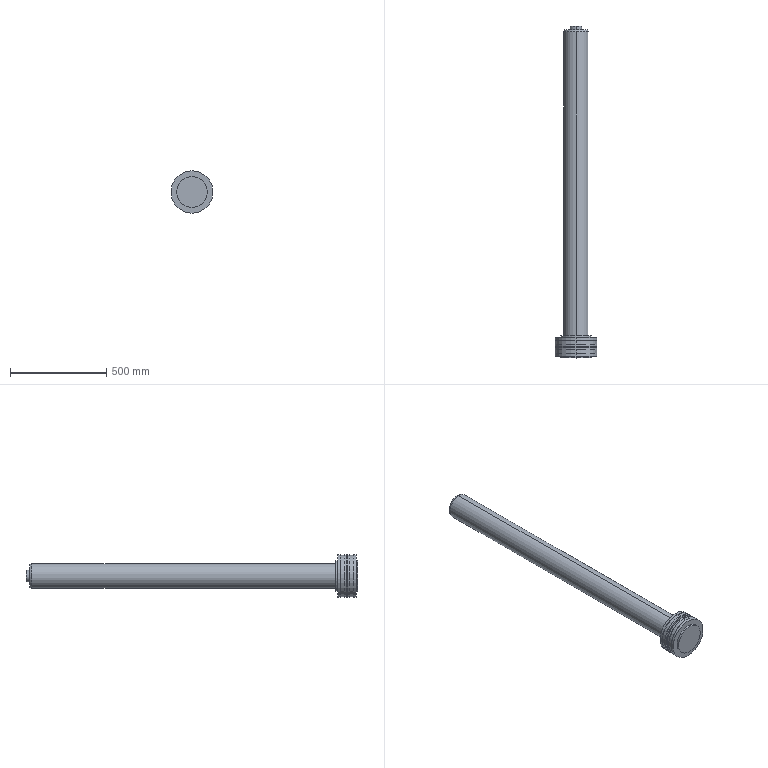Part | SolidWorks | features Revolution 1 | 1 solid | 36 faces | box 220 x 1728 x 220 mm | volume 25109118 mm3 | cylinder 22 | plane 12 | cone 2 | commonest cylinder face diameters 220 x8 160 x4 215 x4 60 x2 130 x2 199 x2
STEP:
#1=CARTESIAN_POINT('',(0.,1728.,-30.));
#2=VERTEX_POINT('',#1);
#3=CARTESIAN_POINT('',(0.,1728.,30.));
#4=VERTEX_POINT('',#3);
#5=CARTESIAN_POINT('',(0.,1728.,0.));
#6=DIRECTION('',(0.,-1.,0.));
#7=DIRECTION('',(0.,0.,-1.));
#8=AXIS2_PLACEMENT_3D('',#5,#6,#7);
#9=CIRCLE('',#8,30.);
#10=EDGE_CURVE('',#2,#4,#9,.T.);
#11=ORIENTED_EDGE('',*,*,#10,.T.);
#12=CARTESIAN_POINT('',(0.,1708.,30.));
#13=VERTEX_POINT('',#12);
#14=CARTESIAN_POINT('',(0.,0.,30.));
#15=DIRECTION('',(0.,-1.,0.));
#16=VECTOR('',#15,1000.);
#17=LINE('',#14,#16);
#18=EDGE_CURVE('',#4,#13,#17,.T.);
#19=ORIENTED_EDGE('',*,*,#18,.T.);
#20=CARTESIAN_POINT('',(0.,1708.,-30.));
#21=VERTEX_POINT('',#20);
#22=CARTESIAN_POINT('',(0.,1708.,0.));
#23=DIRECTION('',(0.,-1.,0.));
#24=DIRECTION('',(0.,0.,-1.));
#25=AXIS2_PLACEMENT_3D('',#22,#23,#24);
#26=CIRCLE('',#25,30.);
#27=EDGE_CURVE('',#21,#13,#26,.T.);
#28=ORIENTED_EDGE('',*,*,#27,.F.);
#29=CARTESIAN_POINT('',(0.,0.,-30.));
#30=DIRECTION('',(0.,-1.,0.));
#31=VECTOR('',#30,1000.);
#32=LINE('',#29,#31);
#33=EDGE_CURVE('',#2,#21,#32,.T.);
#34=ORIENTED_EDGE('',*,*,#33,.F.);
#35=EDGE_LOOP('',(#11,#19,#28,#34));
#36=FACE_OUTER_BOUND('',#35,.T.);
#37=CARTESIAN_POINT('',(0.,0.,0.));
#38=DIRECTION('',(0.,-1.,0.));
#39=DIRECTION('',(0.,0.,-1.));
#40=AXIS2_PLACEMENT_3D('',#37,#38,#39);
#41=CYLINDRICAL_SURFACE('',#40,30.);
#42=ADVANCED_FACE('',(#36),#41,.T.);
#43=CARTESIAN_POINT('',(0.,1708.,-61.36));
#44=VERTEX_POINT('',#43);
#45=CARTESIAN_POINT('',(0.,1708.,61.36));
#46=VERTEX_POINT('',#45);
#47=CARTESIAN_POINT('',(0.,1708.,0.));
#48=DIRECTION('',(0.,-1.,0.));
#49=DIRECTION('',(0.,0.,-1.));
#50=AXIS2_PLACEMENT_3D('',#47,#48,#49);
#51=CIRCLE('',#50,61.36);
#52=EDGE_CURVE('',#44,#46,#51,.T.);
#53=ORIENTED_EDGE('',*,*,#52,.T.);
#54=CARTESIAN_POINT('',(0.,1698.,65.));
#55=VERTEX_POINT('',#54);
#56=CARTESIAN_POINT('',(0.,1698.,65.));
#57=DIRECTION('',(0.,-0.9397,0.342));
#58=VECTOR('',#57,1000.);
#59=LINE('',#56,#58);
#60=EDGE_CURVE('',#46,#55,#59,.T.);
#61=ORIENTED_EDGE('',*,*,#60,.T.);
#62=CARTESIAN_POINT('',(0.,1698.,-65.));
#63=VERTEX_POINT('',#62);
#64=CARTESIAN_POINT('',(0.,1698.,0.));
#65=DIRECTION('',(0.,-1.,0.));
#66=DIRECTION('',(0.,0.,-1.));
#67=AXIS2_PLACEMENT_3D('',#64,#65,#66);
#68=CIRCLE('',#67,65.);
#69=EDGE_CURVE('',#63,#55,#68,.T.);
#70=ORIENTED_EDGE('',*,*,#69,.F.);
#71=CARTESIAN_POINT('',(0.,1698.,-65.));
#72=DIRECTION('',(0.,-0.9397,-0.342));
#73=VECTOR('',#72,1000.);
#74=LINE('',#71,#73);
#75=EDGE_CURVE('',#44,#63,#74,.T.);
#76=ORIENTED_EDGE('',*,*,#75,.F.);
#77=EDGE_LOOP('',(#53,#61,#70,#76));
#78=FACE_OUTER_BOUND('',#77,.T.);
#79=CARTESIAN_POINT('',(0.,1698.,0.));
#80=DIRECTION('',(0.,-1.,0.));
#81=DIRECTION('',(0.,0.,-1.));
#82=AXIS2_PLACEMENT_3D('',#79,#80,#81);
#83=CONICAL_SURFACE('',#82,65.,0.3491);
#84=ADVANCED_FACE('',(#78),#83,.T.);
#85=ORIENTED_EDGE('',*,*,#69,.T.);
#86=CARTESIAN_POINT('',(0.,116.,65.));
#87=VERTEX_POINT('',#86);
#88=CARTESIAN_POINT('',(0.,0.,65.));
#89=DIRECTION('',(0.,-1.,0.));
#90=VECTOR('',#89,1000.);
#91=LINE('',#88,#90);
#92=EDGE_CURVE('',#55,#87,#91,.T.);
#93=ORIENTED_EDGE('',*,*,#92,.T.);
#94=CARTESIAN_POINT('',(0.,116.,-65.));
#95=VERTEX_POINT('',#94);
#96=CARTESIAN_POINT('',(0.,116.,0.));
#97=DIRECTION('',(0.,-1.,0.));
#98=DIRECTION('',(0.,0.,-1.));
#99=AXIS2_PLACEMENT_3D('',#96,#97,#98);
#100=CIRCLE('',#99,65.);
#101=EDGE_CURVE('',#95,#87,#100,.T.);
#102=ORIENTED_EDGE('',*,*,#101,.F.);
#103=CARTESIAN_POINT('',(0.,0.,-65.));
#104=DIRECTION('',(0.,-1.,0.));
#105=VECTOR('',#104,1000.);
#106=LINE('',#103,#105);
#107=EDGE_CURVE('',#63,#95,#106,.T.);
#108=ORIENTED_EDGE('',*,*,#107,.F.);
#109=EDGE_LOOP('',(#85,#93,#102,#108));
#110=FACE_OUTER_BOUND('',#109,.T.);
#111=CARTESIAN_POINT('',(0.,0.,0.));
#112=DIRECTION('',(0.,-1.,0.));
#113=DIRECTION('',(0.,0.,-1.));
#114=AXIS2_PLACEMENT_3D('',#111,#112,#113);
#115=CYLINDRICAL_SURFACE('',#114,65.);
#116=ADVANCED_FACE('',(#110),#115,.T.);
#117=CARTESIAN_POINT('',(0.,116.,-80.));
#118=VERTEX_POINT('',#117);
#119=CARTESIAN_POINT('',(0.,116.,80.));
#120=VERTEX_POINT('',#119);
#121=CARTESIAN_POINT('',(0.,116.,0.));
#122=DIRECTION('',(0.,-1.,0.));
#123=DIRECTION('',(0.,0.,-1.));
#124=AXIS2_PLACEMENT_3D('',#121,#122,#123);
#125=CIRCLE('',#124,80.);
#126=EDGE_CURVE('',#118,#120,#125,.T.);
#127=ORIENTED_EDGE('',*,*,#126,.T.);
#128=CARTESIAN_POINT('',(0.,106.,80.));
#129=VERTEX_POINT('',#128);
#130=CARTESIAN_POINT('',(0.,0.,80.));
#131=DIRECTION('',(0.,-1.,0.));
#132=VECTOR('',#131,1000.);
#133=LINE('',#130,#132);
#134=EDGE_CURVE('',#120,#129,#133,.T.);
#135=ORIENTED_EDGE('',*,*,#134,.T.);
#136=CARTESIAN_POINT('',(0.,106.,-80.));
#137=VERTEX_POINT('',#136);
#138=CARTESIAN_POINT('',(0.,106.,0.));
#139=DIRECTION('',(0.,-1.,0.));
#140=DIRECTION('',(0.,0.,-1.));
#141=AXIS2_PLACEMENT_3D('',#138,#139,#140);
#142=CIRCLE('',#141,80.);
#143=EDGE_CURVE('',#137,#129,#142,.T.);
#144=ORIENTED_EDGE('',*,*,#143,.F.);
#145=CARTESIAN_POINT('',(0.,0.,-80.));
#146=DIRECTION('',(0.,-1.,0.));
#147=VECTOR('',#146,1000.);
#148=LINE('',#145,#147);
#149=EDGE_CURVE('',#118,#137,#148,.T.);
#150=ORIENTED_EDGE('',*,*,#149,.F.);
#151=EDGE_LOOP('',(#127,#135,#144,#150));
#152=FACE_OUTER_BOUND('',#151,.T.);
#153=CARTESIAN_POINT('',(0.,0.,0.));
#154=DIRECTION('',(0.,-1.,0.));
#155=DIRECTION('',(0.,0.,-1.));
#156=AXIS2_PLACEMENT_3D('',#153,#154,#155);
#157=CYLINDRICAL_SURFACE('',#156,80.);
#158=ADVANCED_FACE('',(#152),#157,.T.);
#159=CARTESIAN_POINT('',(0.,106.,-110.));
#160=VERTEX_POINT('',#159);
#161=CARTESIAN_POINT('',(0.,106.,110.));
#162=VERTEX_POINT('',#161);
#163=CARTESIAN_POINT('',(0.,106.,0.));
#164=DIRECTION('',(0.,-1.,0.));
#165=DIRECTION('',(0.,0.,-1.));
#166=AXIS2_PLACEMENT_3D('',#163,#164,#165);
#167=CIRCLE('',#166,110.);
#168=EDGE_CURVE('',#160,#162,#167,.T.);
#169=ORIENTED_EDGE('',*,*,#168,.T.);
#170=CARTESIAN_POINT('',(0.,92.,110.));
#171=VERTEX_POINT('',#170);
#172=CARTESIAN_POINT('',(0.,0.,110.));
#173=DIRECTION('',(0.,-1.,0.));
#174=VECTOR('',#173,1000.);
#175=LINE('',#172,#174);
#176=EDGE_CURVE('',#162,#171,#175,.T.);
#177=ORIENTED_EDGE('',*,*,#176,.T.);
#178=CARTESIAN_POINT('',(0.,92.,-110.));
#179=VERTEX_POINT('',#178);
#180=CARTESIAN_POINT('',(0.,92.,0.));
#181=DIRECTION('',(0.,-1.,0.));
#182=DIRECTION('',(0.,0.,-1.));
#183=AXIS2_PLACEMENT_3D('',#180,#181,#182);
#184=CIRCLE('',#183,110.);
#185=EDGE_CURVE('',#179,#171,#184,.T.);
#186=ORIENTED_EDGE('',*,*,#185,.F.);
#187=CARTESIAN_POINT('',(0.,0.,-110.));
#188=DIRECTION('',(0.,-1.,0.));
#189=VECTOR('',#188,1000.);
#190=LINE('',#187,#189);
#191=EDGE_CURVE('',#160,#179,#190,.T.);
#192=ORIENTED_EDGE('',*,*,#191,.F.);
#193=EDGE_LOOP('',(#169,#177,#186,#192));
#194=FACE_OUTER_BOUND('',#193,.T.);
#195=CARTESIAN_POINT('',(0.,0.,0.));
#196=DIRECTION('',(0.,-1.,0.));
#197=DIRECTION('',(0.,0.,-1.));
#198=AXIS2_PLACEMENT_3D('',#195,#196,#197);
#199=CYLINDRICAL_SURFACE('',#198,110.);
#200=ADVANCED_FACE('',(#194),#199,.T.);
#201=CARTESIAN_POINT('',(0.,92.,-107.5));
#202=VERTEX_POINT('',#201);
#203=CARTESIAN_POINT('',(0.,92.,107.5));
#204=VERTEX_POINT('',#203);
#205=CARTESIAN_POINT('',(0.,92.,0.));
#206=DIRECTION('',(0.,-1.,0.));
#207=DIRECTION('',(0.,0.,-1.));
#208=AXIS2_PLACEMENT_3D('',#205,#206,#207);
#209=CIRCLE('',#208,107.5);
#210=EDGE_CURVE('',#202,#204,#209,.T.);
#211=ORIENTED_EDGE('',*,*,#210,.T.);
#212=CARTESIAN_POINT('',(0.,72.,107.5));
#213=VERTEX_POINT('',#212);
#214=CARTESIAN_POINT('',(0.,0.,107.5));
#215=DIRECTION('',(0.,-1.,0.));
#216=VECTOR('',#215,1000.);
#217=LINE('',#214,#216);
#218=EDGE_CURVE('',#204,#213,#217,.T.);
#219=ORIENTED_EDGE('',*,*,#218,.T.);
#220=CARTESIAN_POINT('',(0.,72.,-107.5));
#221=VERTEX_POINT('',#220);
#222=CARTESIAN_POINT('',(0.,72.,0.));
#223=DIRECTION('',(0.,-1.,0.));
#224=DIRECTION('',(0.,0.,-1.));
#225=AXIS2_PLACEMENT_3D('',#222,#223,#224);
#226=CIRCLE('',#225,107.5);
#227=EDGE_CURVE('',#221,#213,#226,.T.);
#228=ORIENTED_EDGE('',*,*,#227,.F.);
#229=CARTESIAN_POINT('',(0.,0.,-107.5));
#230=DIRECTION('',(0.,-1.,0.));
#231=VECTOR('',#230,1000.);
#232=LINE('',#229,#231);
#233=EDGE_CURVE('',#202,#221,#232,.T.);
#234=ORIENTED_EDGE('',*,*,#233,.F.);
#235=EDGE_LOOP('',(#211,#219,#228,#234));
#236=FACE_OUTER_BOUND('',#235,.T.);
#237=CARTESIAN_POINT('',(0.,0.,0.));
#238=DIRECTION('',(0.,-1.,0.));
#239=DIRECTION('',(0.,0.,-1.));
#240=AXIS2_PLACEMENT_3D('',#237,#238,#239);
#241=CYLINDRICAL_SURFACE('',#240,107.5);
#242=ADVANCED_FACE('',(#236),#241,.T.);
#243=CARTESIAN_POINT('',(0.,72.,-110.));
#244=VERTEX_POINT('',#243);
#245=CARTESIAN_POINT('',(0.,72.,110.));
#246=VERTEX_POINT('',#245);
#247=CARTESIAN_POINT('',(0.,72.,0.));
#248=DIRECTION('',(0.,-1.,0.));
#249=DIRECTION('',(0.,0.,-1.));
#250=AXIS2_PLACEMENT_3D('',#247,#248,#249);
#251=CIRCLE('',#250,110.);
#252=EDGE_CURVE('',#244,#246,#251,.T.);
#253=ORIENTED_EDGE('',*,*,#252,.T.);
#254=CARTESIAN_POINT('',(0.,62.,110.));
#255=VERTEX_POINT('',#254);
#256=CARTESIAN_POINT('',(0.,0.,110.));
#257=DIRECTION('',(0.,-1.,0.));
#258=VECTOR('',#257,1000.);
#259=LINE('',#256,#258);
#260=EDGE_CURVE('',#246,#255,#259,.T.);
#261=ORIENTED_EDGE('',*,*,#260,.T.);
#262=CARTESIAN_POINT('',(0.,62.,-110.));
#263=VERTEX_POINT('',#262);
#264=CARTESIAN_POINT('',(0.,62.,0.));
#265=DIRECTION('',(0.,-1.,0.));
#266=DIRECTION('',(0.,0.,-1.));
#267=AXIS2_PLACEMENT_3D('',#264,#265,#266);
#268=CIRCLE('',#267,110.);
#269=EDGE_CURVE('',#263,#255,#268,.T.);
#270=ORIENTED_EDGE('',*,*,#269,.F.);
#271=CARTESIAN_POINT('',(0.,0.,-110.));
#272=DIRECTION('',(0.,-1.,0.));
#273=VECTOR('',#272,1000.);
#274=LINE('',#271,#273);
#275=EDGE_CURVE('',#244,#263,#274,.T.);
#276=ORIENTED_EDGE('',*,*,#275,.F.);
#277=EDGE_LOOP('',(#253,#261,#270,#276));
#278=FACE_OUTER_BOUND('',#277,.T.);
#279=CARTESIAN_POINT('',(0.,0.,0.));
#280=DIRECTION('',(0.,-1.,0.));
#281=DIRECTION('',(0.,0.,-1.));
#282=AXIS2_PLACEMENT_3D('',#279,#280,#281);
#283=CYLINDRICAL_SURFACE('',#282,110.);
#284=ADVANCED_FACE('',(#278),#283,.T.);
#285=CARTESIAN_POINT('',(0.,62.,-99.5));
#286=VERTEX_POINT('',#285);
#287=CARTESIAN_POINT('',(0.,62.,99.5));
#288=VERTEX_POINT('',#287);
#289=CARTESIAN_POINT('',(0.,62.,0.));
#290=DIRECTION('',(0.,-1.,0.));
#291=DIRECTION('',(0.,0.,-1.));
#292=AXIS2_PLACEMENT_3D('',#289,#290,#291);
#293=CIRCLE('',#292,99.5);
#294=EDGE_CURVE('',#286,#288,#293,.T.);
#295=ORIENTED_EDGE('',*,*,#294,.T.);
#296=CARTESIAN_POINT('',(0.,53.9,99.5));
#297=VERTEX_POINT('',#296);
#298=CARTESIAN_POINT('',(0.,0.,99.5));
#299=DIRECTION('',(0.,-1.,0.));
#300=VECTOR('',#299,1000.);
#301=LINE('',#298,#300);
#302=EDGE_CURVE('',#288,#297,#301,.T.);
#303=ORIENTED_EDGE('',*,*,#302,.T.);
#304=CARTESIAN_POINT('',(0.,53.9,-99.5));
#305=VERTEX_POINT('',#304);
#306=CARTESIAN_POINT('',(0.,53.9,0.));
#307=DIRECTION('',(0.,-1.,0.));
#308=DIRECTION('',(0.,0.,-1.));
#309=AXIS2_PLACEMENT_3D('',#306,#307,#308);
#310=CIRCLE('',#309,99.5);
#311=EDGE_CURVE('',#305,#297,#310,.T.);
#312=ORIENTED_EDGE('',*,*,#311,.F.);
#313=CARTESIAN_POINT('',(0.,0.,-99.5));
#314=DIRECTION('',(0.,-1.,0.));
#315=VECTOR('',#314,1000.);
#316=LINE('',#313,#315);
#317=EDGE_CURVE('',#286,#305,#316,.T.);
#318=ORIENTED_EDGE('',*,*,#317,.F.);
#319=EDGE_LOOP('',(#295,#303,#312,#318));
#320=FACE_OUTER_BOUND('',#319,.T.);
#321=CARTESIAN_POINT('',(0.,0.,0.));
#322=DIRECTION('',(0.,-1.,0.));
#323=DIRECTION('',(0.,0.,-1.));
#324=AXIS2_PLACEMENT_3D('',#321,#322,#323);
#325=CYLINDRICAL_SURFACE('',#324,99.5);
#326=ADVANCED_FACE('',(#320),#325,.T.);
#327=CARTESIAN_POINT('',(0.,53.9,-110.));
#328=VERTEX_POINT('',#327);
#329=CARTESIAN_POINT('',(0.,53.9,110.));
#330=VERTEX_POINT('',#329);
#331=CARTESIAN_POINT('',(0.,53.9,0.));
#332=DIRECTION('',(0.,-1.,0.));
#333=DIRECTION('',(0.,0.,-1.));
#334=AXIS2_PLACEMENT_3D('',#331,#332,#333);
#335=CIRCLE('',#334,110.);
#336=EDGE_CURVE('',#328,#330,#335,.T.);
#337=ORIENTED_EDGE('',*,*,#336,.T.);
#338=CARTESIAN_POINT('',(0.,43.9,110.));
#339=VERTEX_POINT('',#338);
#340=CARTESIAN_POINT('',(0.,0.,110.));
#341=DIRECTION('',(0.,-1.,0.));
#342=VECTOR('',#341,1000.);
#343=LINE('',#340,#342);
#344=EDGE_CURVE('',#330,#339,#343,.T.);
#345=ORIENTED_EDGE('',*,*,#344,.T.);
#346=CARTESIAN_POINT('',(0.,43.9,-110.));
#347=VERTEX_POINT('',#346);
#348=CARTESIAN_POINT('',(0.,43.9,0.));
#349=DIRECTION('',(0.,-1.,0.));
#350=DIRECTION('',(0.,0.,-1.));
#351=AXIS2_PLACEMENT_3D('',#348,#349,#350);
#352=CIRCLE('',#351,110.);
#353=EDGE_CURVE('',#347,#339,#352,.T.);
#354=ORIENTED_EDGE('',*,*,#353,.F.);
#355=CARTESIAN_POINT('',(0.,0.,-110.));
#356=DIRECTION('',(0.,-1.,0.));
#357=VECTOR('',#356,1000.);
#358=LINE('',#355,#357);
#359=EDGE_CURVE('',#328,#347,#358,.T.);
#360=ORIENTED_EDGE('',*,*,#359,.F.);
#361=EDGE_LOOP('',(#337,#345,#354,#360));
#362=FACE_OUTER_BOUND('',#361,.T.);
#363=CARTESIAN_POINT('',(0.,0.,0.));
#364=DIRECTION('',(0.,-1.,0.));
#365=DIRECTION('',(0.,0.,-1.));
#366=AXIS2_PLACEMENT_3D('',#363,#364,#365);
#367=CYLINDRICAL_SURFACE('',#366,110.);
#368=ADVANCED_FACE('',(#362),#367,.T.);
#369=CARTESIAN_POINT('',(0.,43.9,-107.5));
#370=VERTEX_POINT('',#369);
#371=CARTESIAN_POINT('',(0.,43.9,107.5));
#372=VERTEX_POINT('',#371);
#373=CARTESIAN_POINT('',(0.,43.9,0.));
#374=DIRECTION('',(0.,-1.,0.));
#375=DIRECTION('',(0.,0.,-1.));
#376=AXIS2_PLACEMENT_3D('',#373,#374,#375);
#377=CIRCLE('',#376,107.5);
#378=EDGE_CURVE('',#370,#372,#377,.T.);
#379=ORIENTED_EDGE('',*,*,#378,.T.);
#380=CARTESIAN_POINT('',(0.,23.9,107.5));
#381=VERTEX_POINT('',#380);
#382=CARTESIAN_POINT('',(0.,0.,107.5));
#383=DIRECTION('',(0.,-1.,0.));
#384=VECTOR('',#383,1000.);
#385=LINE('',#382,#384);
#386=EDGE_CURVE('',#372,#381,#385,.T.);
#387=ORIENTED_EDGE('',*,*,#386,.T.);
#388=CARTESIAN_POINT('',(0.,23.9,-107.5));
#389=VERTEX_POINT('',#388);
#390=CARTESIAN_POINT('',(0.,23.9,0.));
#391=DIRECTION('',(0.,-1.,0.));
#392=DIRECTION('',(0.,0.,-1.));
#393=AXIS2_PLACEMENT_3D('',#390,#391,#392);
#394=CIRCLE('',#393,107.5);
#395=EDGE_CURVE('',#389,#381,#394,.T.);
#396=ORIENTED_EDGE('',*,*,#395,.F.);
#397=CARTESIAN_POINT('',(0.,0.,-107.5));
#398=DIRECTION('',(0.,-1.,0.));
#399=VECTOR('',#398,1000.);
#400=LINE('',#397,#399);
#401=EDGE_CURVE('',#370,#389,#400,.T.);
#402=ORIENTED_EDGE('',*,*,#401,.F.);
#403=EDGE_LOOP('',(#379,#387,#396,#402));
#404=FACE_OUTER_BOUND('',#403,.T.);
#405=CARTESIAN_POINT('',(0.,0.,0.));
#406=DIRECTION('',(0.,-1.,0.));
#407=DIRECTION('',(0.,0.,-1.));
#408=AXIS2_PLACEMENT_3D('',#405,#406,#407);
#409=CYLINDRICAL_SURFACE('',#408,107.5);
#410=ADVANCED_FACE('',(#404),#409,.T.);
#411=CARTESIAN_POINT('',(0.,23.9,-110.));
#412=VERTEX_POINT('',#411);
#413=CARTESIAN_POINT('',(0.,23.9,110.));
#414=VERTEX_POINT('',#413);
#415=CARTESIAN_POINT('',(0.,23.9,0.));
#416=DIRECTION('',(0.,-1.,0.));
#417=DIRECTION('',(0.,0.,-1.));
#418=AXIS2_PLACEMENT_3D('',#415,#416,#417);
#419=CIRCLE('',#418,110.);
#420=EDGE_CURVE('',#412,#414,#419,.T.);
#421=ORIENTED_EDGE('',*,*,#420,.T.);
#422=CARTESIAN_POINT('',(0.,9.9,110.));
#423=VERTEX_POINT('',#422);
#424=CARTESIAN_POINT('',(0.,0.,110.));
#425=DIRECTION('',(0.,-1.,0.));
#426=VECTOR('',#425,1000.);
#427=LINE('',#424,#426);
#428=EDGE_CURVE('',#414,#423,#427,.T.);
#429=ORIENTED_EDGE('',*,*,#428,.T.);
#430=CARTESIAN_POINT('',(0.,9.9,-110.));
#431=VERTEX_POINT('',#430);
#432=CARTESIAN_POINT('',(0.,9.9,0.));
#433=DIRECTION('',(0.,-1.,0.));
#434=DIRECTION('',(0.,0.,-1.));
#435=AXIS2_PLACEMENT_3D('',#432,#433,#434);
#436=CIRCLE('',#435,110.);
#437=EDGE_CURVE('',#431,#423,#436,.T.);
#438=ORIENTED_EDGE('',*,*,#437,.F.);
#439=CARTESIAN_POINT('',(0.,0.,-110.));
#440=DIRECTION('',(0.,-1.,0.));
#441=VECTOR('',#440,1000.);
#442=LINE('',#439,#441);
#443=EDGE_CURVE('',#412,#431,#442,.T.);
#444=ORIENTED_EDGE('',*,*,#443,.F.);
#445=EDGE_LOOP('',(#421,#429,#438,#444));
#446=FACE_OUTER_BOUND('',#445,.T.);
#447=CARTESIAN_POINT('',(0.,0.,0.));
#448=DIRECTION('',(0.,-1.,0.));
#449=DIRECTION('',(0.,0.,-1.));
#450=AXIS2_PLACEMENT_3D('',#447,#448,#449);
#451=CYLINDRICAL_SURFACE('',#450,110.);
#452=ADVANCED_FACE('',(#446),#451,.T.);
#453=CARTESIAN_POINT('',(0.,9.9,-80.));
#454=VERTEX_POINT('',#453);
#455=CARTESIAN_POINT('',(0.,9.9,80.));
#456=VERTEX_POINT('',#455);
#457=CARTESIAN_POINT('',(0.,9.9,0.));
#458=DIRECTION('',(0.,-1.,0.));
#459=DIRECTION('',(0.,0.,-1.));
#460=AXIS2_PLACEMENT_3D('',#457,#458,#459);
#461=CIRCLE('',#460,80.);
#462=EDGE_CURVE('',#454,#456,#461,.T.);
#463=ORIENTED_EDGE('',*,*,#462,.T.);
#464=CARTESIAN_POINT('',(0.,0.,80.));
#465=VERTEX_POINT('',#464);
#466=CARTESIAN_POINT('',(0.,0.,80.));
#467=DIRECTION('',(0.,-1.,0.));
#468=VECTOR('',#467,1000.);
#469=LINE('',#466,#468);
#470=EDGE_CURVE('',#456,#465,#469,.T.);
#471=ORIENTED_EDGE('',*,*,#470,.T.);
#472=CARTESIAN_POINT('',(0.,0.,-80.));
#473=VERTEX_POINT('',#472);
#474=CARTESIAN_POINT('',(0.,0.,0.));
#475=DIRECTION('',(0.,-1.,0.));
#476=DIRECTION('',(0.,0.,-1.));
#477=AXIS2_PLACEMENT_3D('',#474,#475,#476);
#478=CIRCLE('',#477,80.);
#479=EDGE_CURVE('',#473,#465,#478,.T.);
#480=ORIENTED_EDGE('',*,*,#479,.F.);
#481=CARTESIAN_POINT('',(0.,0.,-80.));
#482=DIRECTION('',(0.,-1.,0.));
#483=VECTOR('',#482,1000.);
#484=LINE('',#481,#483);
#485=EDGE_CURVE('',#454,#473,#484,.T.);
#486=ORIENTED_EDGE('',*,*,#485,.F.);
#487=EDGE_LOOP('',(#463,#471,#480,#486));
#488=FACE_OUTER_BOUND('',#487,.T.);
#489=CARTESIAN_POINT('',(0.,0.,0.));
#490=DIRECTION('',(0.,-1.,0.));
#491=DIRECTION('',(0.,0.,-1.));
#492=AXIS2_PLACEMENT_3D('',#489,#490,#491);
#493=CYLINDRICAL_SURFACE('',#492,80.);
#494=ADVANCED_FACE('',(#488),#493,.T.);
#495=ORIENTED_EDGE('',*,*,#479,.T.);
#496=CARTESIAN_POINT('',(0.,0.,0.));
#497=DIRECTION('',(0.,-1.,0.));
#498=DIRECTION('',(0.,0.,-1.));
#499=AXIS2_PLACEMENT_3D('',#496,#497,#498);
#500=CIRCLE('',#499,80.);
#501=EDGE_CURVE('',#465,#473,#500,.T.);
#502=ORIENTED_EDGE('',*,*,#501,.T.);
#503=EDGE_LOOP('',(#495,#502));
#504=FACE_OUTER_BOUND('',#503,.T.);
#505=CARTESIAN_POINT('',(0.,0.,0.));
#506=DIRECTION('',(0.,-1.,0.));
#507=DIRECTION('',(0.,0.,-1.));
#508=AXIS2_PLACEMENT_3D('',#505,#506,#507);
#509=PLANE('',#508);
#510=ADVANCED_FACE('',(#504),#509,.T.);
#511=ORIENTED_EDGE('',*,*,#470,.F.);
#512=CARTESIAN_POINT('',(0.,9.9,0.));
#513=DIRECTION('',(0.,-1.,0.));
#514=DIRECTION('',(0.,0.,-1.));
#515=AXIS2_PLACEMENT_3D('',#512,#513,#514);
#516=CIRCLE('',#515,80.);
#517=EDGE_CURVE('',#456,#454,#516,.T.);
#518=ORIENTED_EDGE('',*,*,#517,.T.);
#519=ORIENTED_EDGE('',*,*,#485,.T.);
#520=ORIENTED_EDGE('',*,*,#501,.F.);
#521=EDGE_LOOP('',(#511,#518,#519,#520));
#522=FACE_OUTER_BOUND('',#521,.T.);
#523=CARTESIAN_POINT('',(0.,0.,0.));
#524=DIRECTION('',(0.,-1.,0.));
#525=DIRECTION('',(0.,0.,-1.));
#526=AXIS2_PLACEMENT_3D('',#523,#524,#525);
#527=CYLINDRICAL_SURFACE('',#526,80.);
#528=ADVANCED_FACE('',(#522),#527,.T.);
#529=ORIENTED_EDGE('',*,*,#437,.T.);
#530=CARTESIAN_POINT('',(0.,9.9,0.));
#531=DIRECTION('',(0.,-1.,0.));
#532=DIRECTION('',(0.,0.,-1.));
#533=AXIS2_PLACEMENT_3D('',#530,#531,#532);
#534=CIRCLE('',#533,110.);
#535=EDGE_CURVE('',#423,#431,#534,.T.);
#536=ORIENTED_EDGE('',*,*,#535,.T.);
#537=EDGE_LOOP('',(#529,#536));
#538=FACE_OUTER_BOUND('',#537,.T.);
#539=ORIENTED_EDGE('',*,*,#462,.F.);
#540=ORIENTED_EDGE('',*,*,#517,.F.);
#541=EDGE_LOOP('',(#539,#540));
#542=FACE_BOUND('',#541,.T.);
#543=CARTESIAN_POINT('',(80.,9.9,0.));
#544=DIRECTION('',(0.,-1.,0.));
#545=DIRECTION('',(0.,0.,-1.));
#546=AXIS2_PLACEMENT_3D('',#543,#544,#545);
#547=PLANE('',#546);
#548=ADVANCED_FACE('',(#538,#542),#547,.T.);
#549=ORIENTED_EDGE('',*,*,#428,.F.);
#550=CARTESIAN_POINT('',(0.,23.9,0.));
#551=DIRECTION('',(0.,-1.,0.));
#552=DIRECTION('',(0.,0.,-1.));
#553=AXIS2_PLACEMENT_3D('',#550,#551,#552);
#554=CIRCLE('',#553,110.);
#555=EDGE_CURVE('',#414,#412,#554,.T.);
#556=ORIENTED_EDGE('',*,*,#555,.T.);
#557=ORIENTED_EDGE('',*,*,#443,.T.);
#558=ORIENTED_EDGE('',*,*,#535,.F.);
#559=EDGE_LOOP('',(#549,#556,#557,#558));
#560=FACE_OUTER_BOUND('',#559,.T.);
#561=CARTESIAN_POINT('',(0.,0.,0.));
#562=DIRECTION('',(0.,-1.,0.));
#563=DIRECTION('',(0.,0.,-1.));
#564=AXIS2_PLACEMENT_3D('',#561,#562,#563);
#565=CYLINDRICAL_SURFACE('',#564,110.);
#566=ADVANCED_FACE('',(#560),#565,.T.);
#567=ORIENTED_EDGE('',*,*,#395,.T.);
#568=CARTESIAN_POINT('',(0.,23.9,0.));
#569=DIRECTION('',(0.,-1.,0.));
#570=DIRECTION('',(0.,0.,-1.));
#571=AXIS2_PLACEMENT_3D('',#568,#569,#570);
#572=CIRCLE('',#571,107.5);
#573=EDGE_CURVE('',#381,#389,#572,.T.);
#574=ORIENTED_EDGE('',*,*,#573,.T.);
#575=EDGE_LOOP('',(#567,#574));
#576=FACE_BOUND('',#575,.T.);
#577=ORIENTED_EDGE('',*,*,#420,.F.);
#578=ORIENTED_EDGE('',*,*,#555,.F.);
#579=EDGE_LOOP('',(#577,#578));
#580=FACE_OUTER_BOUND('',#579,.T.);
#581=CARTESIAN_POINT('',(110.,23.9,0.));
#582=DIRECTION('',(0.,1.,0.));
#583=DIRECTION('',(0.,0.,1.));
#584=AXIS2_PLACEMENT_3D('',#581,#582,#583);
#585=PLANE('',#584);
#586=ADVANCED_FACE('',(#576,#580),#585,.T.);
#587=ORIENTED_EDGE('',*,*,#386,.F.);
#588=CARTESIAN_POINT('',(0.,43.9,0.));
#589=DIRECTION('',(0.,-1.,0.));
#590=DIRECTION('',(0.,0.,-1.));
#591=AXIS2_PLACEMENT_3D('',#588,#589,#590);
#592=CIRCLE('',#591,107.5);
#593=EDGE_CURVE('',#372,#370,#592,.T.);
#594=ORIENTED_EDGE('',*,*,#593,.T.);
#595=ORIENTED_EDGE('',*,*,#401,.T.);
#596=ORIENTED_EDGE('',*,*,#573,.F.);
#597=EDGE_LOOP('',(#587,#594,#595,#596));
#598=FACE_OUTER_BOUND('',#597,.T.);
#599=CARTESIAN_POINT('',(0.,0.,0.));
#600=DIRECTION('',(0.,-1.,0.));
#601=DIRECTION('',(0.,0.,-1.));
#602=AXIS2_PLACEMENT_3D('',#599,#600,#601);
#603=CYLINDRICAL_SURFACE('',#602,107.5);
#604=ADVANCED_FACE('',(#598),#603,.T.);
#605=ORIENTED_EDGE('',*,*,#353,.T.);
#606=CARTESIAN_POINT('',(0.,43.9,0.));
#607=DIRECTION('',(0.,-1.,0.));
#608=DIRECTION('',(0.,0.,-1.));
#609=AXIS2_PLACEMENT_3D('',#606,#607,#608);
#610=CIRCLE('',#609,110.);
#611=EDGE_CURVE('',#339,#347,#610,.T.);
#612=ORIENTED_EDGE('',*,*,#611,.T.);
#613=EDGE_LOOP('',(#605,#612));
#614=FACE_OUTER_BOUND('',#613,.T.);
#615=ORIENTED_EDGE('',*,*,#378,.F.);
#616=ORIENTED_EDGE('',*,*,#593,.F.);
#617=EDGE_LOOP('',(#615,#616));
#618=FACE_BOUND('',#617,.T.);
#619=CARTESIAN_POINT('',(107.5,43.9,0.));
#620=DIRECTION('',(0.,-1.,0.));
#621=DIRECTION('',(0.,0.,-1.));
#622=AXIS2_PLACEMENT_3D('',#619,#620,#621);
#623=PLANE('',#622);
#624=ADVANCED_FACE('',(#614,#618),#623,.T.);
#625=ORIENTED_EDGE('',*,*,#344,.F.);
#626=CARTESIAN_POINT('',(0.,53.9,0.));
#627=DIRECTION('',(0.,-1.,0.));
#628=DIRECTION('',(0.,0.,-1.));
#629=AXIS2_PLACEMENT_3D('',#626,#627,#628);
#630=CIRCLE('',#629,110.);
#631=EDGE_CURVE('',#330,#328,#630,.T.);
#632=ORIENTED_EDGE('',*,*,#631,.T.);
#633=ORIENTED_EDGE('',*,*,#359,.T.);
#634=ORIENTED_EDGE('',*,*,#611,.F.);
#635=EDGE_LOOP('',(#625,#632,#633,#634));
#636=FACE_OUTER_BOUND('',#635,.T.);
#637=CARTESIAN_POINT('',(0.,0.,0.));
#638=DIRECTION('',(0.,-1.,0.));
#639=DIRECTION('',(0.,0.,-1.));
#640=AXIS2_PLACEMENT_3D('',#637,#638,#639);
#641=CYLINDRICAL_SURFACE('',#640,110.);
#642=ADVANCED_FACE('',(#636),#641,.T.);
#643=ORIENTED_EDGE('',*,*,#311,.T.);
#644=CARTESIAN_POINT('',(0.,53.9,0.));
#645=DIRECTION('',(0.,-1.,0.));
#646=DIRECTION('',(0.,0.,-1.));
#647=AXIS2_PLACEMENT_3D('',#644,#645,#646);
#648=CIRCLE('',#647,99.5);
#649=EDGE_CURVE('',#297,#305,#648,.T.);
#650=ORIENTED_EDGE('',*,*,#649,.T.);
#651=EDGE_LOOP('',(#643,#650));
#652=FACE_BOUND('',#651,.T.);
#653=ORIENTED_EDGE('',*,*,#336,.F.);
#654=ORIENTED_EDGE('',*,*,#631,.F.);
#655=EDGE_LOOP('',(#653,#654));
#656=FACE_OUTER_BOUND('',#655,.T.);
#657=CARTESIAN_POINT('',(110.,53.9,0.));
#658=DIRECTION('',(0.,1.,0.));
#659=DIRECTION('',(0.,0.,1.));
#660=AXIS2_PLACEMENT_3D('',#657,#658,#659);
#661=PLANE('',#660);
#662=ADVANCED_FACE('',(#652,#656),#661,.T.);
#663=ORIENTED_EDGE('',*,*,#302,.F.);
#664=CARTESIAN_POINT('',(0.,62.,0.));
#665=DIRECTION('',(0.,-1.,0.));
#666=DIRECTION('',(0.,0.,-1.));
#667=AXIS2_PLACEMENT_3D('',#664,#665,#666);
#668=CIRCLE('',#667,99.5);
#669=EDGE_CURVE('',#288,#286,#668,.T.);
#670=ORIENTED_EDGE('',*,*,#669,.T.);
#671=ORIENTED_EDGE('',*,*,#317,.T.);
#672=ORIENTED_EDGE('',*,*,#649,.F.);
#673=EDGE_LOOP('',(#663,#670,#671,#672));
#674=FACE_OUTER_BOUND('',#673,.T.);
#675=CARTESIAN_POINT('',(0.,0.,0.));
#676=DIRECTION('',(0.,-1.,0.));
#677=DIRECTION('',(0.,0.,-1.));
#678=AXIS2_PLACEMENT_3D('',#675,#676,#677);
#679=CYLINDRICAL_SURFACE('',#678,99.5);
#680=ADVANCED_FACE('',(#674),#679,.T.);
#681=ORIENTED_EDGE('',*,*,#269,.T.);
#682=CARTESIAN_POINT('',(0.,62.,0.));
#683=DIRECTION('',(0.,-1.,0.));
#684=DIRECTION('',(0.,0.,-1.));
#685=AXIS2_PLACEMENT_3D('',#682,#683,#684);
#686=CIRCLE('',#685,110.);
#687=EDGE_CURVE('',#255,#263,#686,.T.);
#688=ORIENTED_EDGE('',*,*,#687,.T.);
#689=EDGE_LOOP('',(#681,#688));
#690=FACE_OUTER_BOUND('',#689,.T.);
#691=ORIENTED_EDGE('',*,*,#294,.F.);
#692=ORIENTED_EDGE('',*,*,#669,.F.);
#693=EDGE_LOOP('',(#691,#692));
#694=FACE_BOUND('',#693,.T.);
#695=CARTESIAN_POINT('',(99.5,62.,0.));
#696=DIRECTION('',(0.,-1.,0.));
#697=DIRECTION('',(0.,0.,-1.));
#698=AXIS2_PLACEMENT_3D('',#695,#696,#697);
#699=PLANE('',#698);
#700=ADVANCED_FACE('',(#690,#694),#699,.T.);
#701=ORIENTED_EDGE('',*,*,#260,.F.);
#702=CARTESIAN_POINT('',(0.,72.,0.));
#703=DIRECTION('',(0.,-1.,0.));
#704=DIRECTION('',(0.,0.,-1.));
#705=AXIS2_PLACEMENT_3D('',#702,#703,#704);
#706=CIRCLE('',#705,110.);
#707=EDGE_CURVE('',#246,#244,#706,.T.);
#708=ORIENTED_EDGE('',*,*,#707,.T.);
#709=ORIENTED_EDGE('',*,*,#275,.T.);
#710=ORIENTED_EDGE('',*,*,#687,.F.);
#711=EDGE_LOOP('',(#701,#708,#709,#710));
#712=FACE_OUTER_BOUND('',#711,.T.);
#713=CARTESIAN_POINT('',(0.,0.,0.));
#714=DIRECTION('',(0.,-1.,0.));
#715=DIRECTION('',(0.,0.,-1.));
#716=AXIS2_PLACEMENT_3D('',#713,#714,#715);
#717=CYLINDRICAL_SURFACE('',#716,110.);
#718=ADVANCED_FACE('',(#712),#717,.T.);
#719=ORIENTED_EDGE('',*,*,#227,.T.);
#720=CARTESIAN_POINT('',(0.,72.,0.));
#721=DIRECTION('',(0.,-1.,0.));
#722=DIRECTION('',(0.,0.,-1.));
#723=AXIS2_PLACEMENT_3D('',#720,#721,#722);
#724=CIRCLE('',#723,107.5);
#725=EDGE_CURVE('',#213,#221,#724,.T.);
#726=ORIENTED_EDGE('',*,*,#725,.T.);
#727=EDGE_LOOP('',(#719,#726));
#728=FACE_BOUND('',#727,.T.);
#729=ORIENTED_EDGE('',*,*,#252,.F.);
#730=ORIENTED_EDGE('',*,*,#707,.F.);
#731=EDGE_LOOP('',(#729,#730));
#732=FACE_OUTER_BOUND('',#731,.T.);
#733=CARTESIAN_POINT('',(110.,72.,0.));
#734=DIRECTION('',(0.,1.,0.));
#735=DIRECTION('',(0.,0.,1.));
#736=AXIS2_PLACEMENT_3D('',#733,#734,#735);
#737=PLANE('',#736);
#738=ADVANCED_FACE('',(#728,#732),#737,.T.);
#739=ORIENTED_EDGE('',*,*,#218,.F.);
#740=CARTESIAN_POINT('',(0.,92.,0.));
#741=DIRECTION('',(0.,-1.,0.));
#742=DIRECTION('',(0.,0.,-1.));
#743=AXIS2_PLACEMENT_3D('',#740,#741,#742);
#744=CIRCLE('',#743,107.5);
#745=EDGE_CURVE('',#204,#202,#744,.T.);
#746=ORIENTED_EDGE('',*,*,#745,.T.);
#747=ORIENTED_EDGE('',*,*,#233,.T.);
#748=ORIENTED_EDGE('',*,*,#725,.F.);
#749=EDGE_LOOP('',(#739,#746,#747,#748));
#750=FACE_OUTER_BOUND('',#749,.T.);
#751=CARTESIAN_POINT('',(0.,0.,0.));
#752=DIRECTION('',(0.,-1.,0.));
#753=DIRECTION('',(0.,0.,-1.));
#754=AXIS2_PLACEMENT_3D('',#751,#752,#753);
#755=CYLINDRICAL_SURFACE('',#754,107.5);
#756=ADVANCED_FACE('',(#750),#755,.T.);
#757=ORIENTED_EDGE('',*,*,#185,.T.);
#758=CARTESIAN_POINT('',(0.,92.,0.));
#759=DIRECTION('',(0.,-1.,0.));
#760=DIRECTION('',(0.,0.,-1.));
#761=AXIS2_PLACEMENT_3D('',#758,#759,#760);
#762=CIRCLE('',#761,110.);
#763=EDGE_CURVE('',#171,#179,#762,.T.);
#764=ORIENTED_EDGE('',*,*,#763,.T.);
#765=EDGE_LOOP('',(#757,#764));
#766=FACE_OUTER_BOUND('',#765,.T.);
#767=ORIENTED_EDGE('',*,*,#210,.F.);
#768=ORIENTED_EDGE('',*,*,#745,.F.);
#769=EDGE_LOOP('',(#767,#768));
#770=FACE_BOUND('',#769,.T.);
#771=CARTESIAN_POINT('',(107.5,92.,0.));
#772=DIRECTION('',(0.,-1.,0.));
#773=DIRECTION('',(0.,0.,-1.));
#774=AXIS2_PLACEMENT_3D('',#771,#772,#773);
#775=PLANE('',#774);
#776=ADVANCED_FACE('',(#766,#770),#775,.T.);
#777=ORIENTED_EDGE('',*,*,#176,.F.);
#778=CARTESIAN_POINT('',(0.,106.,0.));
#779=DIRECTION('',(0.,-1.,0.));
#780=DIRECTION('',(0.,0.,-1.));
#781=AXIS2_PLACEMENT_3D('',#778,#779,#780);
#782=CIRCLE('',#781,110.);
#783=EDGE_CURVE('',#162,#160,#782,.T.);
#784=ORIENTED_EDGE('',*,*,#783,.T.);
#785=ORIENTED_EDGE('',*,*,#191,.T.);
#786=ORIENTED_EDGE('',*,*,#763,.F.);
#787=EDGE_LOOP('',(#777,#784,#785,#786));
#788=FACE_OUTER_BOUND('',#787,.T.);
#789=CARTESIAN_POINT('',(0.,0.,0.));
#790=DIRECTION('',(0.,-1.,0.));
#791=DIRECTION('',(0.,0.,-1.));
#792=AXIS2_PLACEMENT_3D('',#789,#790,#791);
#793=CYLINDRICAL_SURFACE('',#792,110.);
#794=ADVANCED_FACE('',(#788),#793,.T.);
#795=ORIENTED_EDGE('',*,*,#143,.T.);
#796=CARTESIAN_POINT('',(0.,106.,0.));
#797=DIRECTION('',(0.,-1.,0.));
#798=DIRECTION('',(0.,0.,-1.));
#799=AXIS2_PLACEMENT_3D('',#796,#797,#798);
#800=CIRCLE('',#799,80.);
#801=EDGE_CURVE('',#129,#137,#800,.T.);
#802=ORIENTED_EDGE('',*,*,#801,.T.);
#803=EDGE_LOOP('',(#795,#802));
#804=FACE_BOUND('',#803,.T.);
#805=ORIENTED_EDGE('',*,*,#168,.F.);
#806=ORIENTED_EDGE('',*,*,#783,.F.);
#807=EDGE_LOOP('',(#805,#806));
#808=FACE_OUTER_BOUND('',#807,.T.);
#809=CARTESIAN_POINT('',(110.,106.,0.));
#810=DIRECTION('',(0.,1.,0.));
#811=DIRECTION('',(0.,0.,1.));
#812=AXIS2_PLACEMENT_3D('',#809,#810,#811);
#813=PLANE('',#812);
#814=ADVANCED_FACE('',(#804,#808),#813,.T.);
#815=ORIENTED_EDGE('',*,*,#134,.F.);
#816=CARTESIAN_POINT('',(0.,116.,0.));
#817=DIRECTION('',(0.,-1.,0.));
#818=DIRECTION('',(0.,0.,-1.));
#819=AXIS2_PLACEMENT_3D('',#816,#817,#818);
#820=CIRCLE('',#819,80.);
#821=EDGE_CURVE('',#120,#118,#820,.T.);
#822=ORIENTED_EDGE('',*,*,#821,.T.);
#823=ORIENTED_EDGE('',*,*,#149,.T.);
#824=ORIENTED_EDGE('',*,*,#801,.F.);
#825=EDGE_LOOP('',(#815,#822,#823,#824));
#826=FACE_OUTER_BOUND('',#825,.T.);
#827=CARTESIAN_POINT('',(0.,0.,0.));
#828=DIRECTION('',(0.,-1.,0.));
#829=DIRECTION('',(0.,0.,-1.));
#830=AXIS2_PLACEMENT_3D('',#827,#828,#829);
#831=CYLINDRICAL_SURFACE('',#830,80.);
#832=ADVANCED_FACE('',(#826),#831,.T.);
#833=ORIENTED_EDGE('',*,*,#101,.T.);
#834=CARTESIAN_POINT('',(0.,116.,0.));
#835=DIRECTION('',(0.,-1.,0.));
#836=DIRECTION('',(0.,0.,-1.));
#837=AXIS2_PLACEMENT_3D('',#834,#835,#836);
#838=CIRCLE('',#837,65.);
#839=EDGE_CURVE('',#87,#95,#838,.T.);
#840=ORIENTED_EDGE('',*,*,#839,.T.);
#841=EDGE_LOOP('',(#833,#840));
#842=FACE_BOUND('',#841,.T.);
#843=ORIENTED_EDGE('',*,*,#126,.F.);
#844=ORIENTED_EDGE('',*,*,#821,.F.);
#845=EDGE_LOOP('',(#843,#844));
#846=FACE_OUTER_BOUND('',#845,.T.);
#847=CARTESIAN_POINT('',(65.,116.,0.));
#848=DIRECTION('',(0.,1.,0.));
#849=DIRECTION('',(0.,0.,1.));
#850=AXIS2_PLACEMENT_3D('',#847,#848,#849);
#851=PLANE('',#850);
#852=ADVANCED_FACE('',(#842,#846),#851,.T.);
#853=ORIENTED_EDGE('',*,*,#92,.F.);
#854=CARTESIAN_POINT('',(0.,1698.,0.));
#855=DIRECTION('',(0.,-1.,0.));
#856=DIRECTION('',(0.,0.,-1.));
#857=AXIS2_PLACEMENT_3D('',#854,#855,#856);
#858=CIRCLE('',#857,65.);
#859=EDGE_CURVE('',#55,#63,#858,.T.);
#860=ORIENTED_EDGE('',*,*,#859,.T.);
#861=ORIENTED_EDGE('',*,*,#107,.T.);
#862=ORIENTED_EDGE('',*,*,#839,.F.);
#863=EDGE_LOOP('',(#853,#860,#861,#862));
#864=FACE_OUTER_BOUND('',#863,.T.);
#865=CARTESIAN_POINT('',(0.,0.,0.));
#866=DIRECTION('',(0.,-1.,0.));
#867=DIRECTION('',(0.,0.,-1.));
#868=AXIS2_PLACEMENT_3D('',#865,#866,#867);
#869=CYLINDRICAL_SURFACE('',#868,65.);
#870=ADVANCED_FACE('',(#864),#869,.T.);
#871=ORIENTED_EDGE('',*,*,#60,.F.);
#872=CARTESIAN_POINT('',(0.,1708.,0.));
#873=DIRECTION('',(0.,-1.,0.));
#874=DIRECTION('',(0.,0.,-1.));
#875=AXIS2_PLACEMENT_3D('',#872,#873,#874);
#876=CIRCLE('',#875,61.36);
#877=EDGE_CURVE('',#46,#44,#876,.T.);
#878=ORIENTED_EDGE('',*,*,#877,.T.);
#879=ORIENTED_EDGE('',*,*,#75,.T.);
#880=ORIENTED_EDGE('',*,*,#859,.F.);
#881=EDGE_LOOP('',(#871,#878,#879,#880));
#882=FACE_OUTER_BOUND('',#881,.T.);
#883=CARTESIAN_POINT('',(0.,1698.,0.));
#884=DIRECTION('',(0.,-1.,0.));
#885=DIRECTION('',(0.,0.,-1.));
#886=AXIS2_PLACEMENT_3D('',#883,#884,#885);
#887=CONICAL_SURFACE('',#886,65.,0.3491);
#888=ADVANCED_FACE('',(#882),#887,.T.);
#889=ORIENTED_EDGE('',*,*,#27,.T.);
#890=CARTESIAN_POINT('',(0.,1708.,0.));
#891=DIRECTION('',(0.,-1.,0.));
#892=DIRECTION('',(0.,0.,-1.));
#893=AXIS2_PLACEMENT_3D('',#890,#891,#892);
#894=CIRCLE('',#893,30.);
#895=EDGE_CURVE('',#13,#21,#894,.T.);
#896=ORIENTED_EDGE('',*,*,#895,.T.);
#897=EDGE_LOOP('',(#889,#896));
#898=FACE_BOUND('',#897,.T.);
#899=ORIENTED_EDGE('',*,*,#52,.F.);
#900=ORIENTED_EDGE('',*,*,#877,.F.);
#901=EDGE_LOOP('',(#899,#900));
#902=FACE_OUTER_BOUND('',#901,.T.);
#903=CARTESIAN_POINT('',(61.36,1708.,0.));
#904=DIRECTION('',(0.,1.,0.));
#905=DIRECTION('',(0.,0.,1.));
#906=AXIS2_PLACEMENT_3D('',#903,#904,#905);
#907=PLANE('',#906);
#908=ADVANCED_FACE('',(#898,#902),#907,.T.);
#909=ORIENTED_EDGE('',*,*,#18,.F.);
#910=CARTESIAN_POINT('',(0.,1728.,0.));
#911=DIRECTION('',(0.,-1.,0.));
#912=DIRECTION('',(0.,0.,-1.));
#913=AXIS2_PLACEMENT_3D('',#910,#911,#912);
#914=CIRCLE('',#913,30.);
#915=EDGE_CURVE('',#4,#2,#914,.T.);
#916=ORIENTED_EDGE('',*,*,#915,.T.);
#917=ORIENTED_EDGE('',*,*,#33,.T.);
#918=ORIENTED_EDGE('',*,*,#895,.F.);
#919=EDGE_LOOP('',(#909,#916,#917,#918));
#920=FACE_OUTER_BOUND('',#919,.T.);
#921=CARTESIAN_POINT('',(0.,0.,0.));
#922=DIRECTION('',(0.,-1.,0.));
#923=DIRECTION('',(0.,0.,-1.));
#924=AXIS2_PLACEMENT_3D('',#921,#922,#923);
#925=CYLINDRICAL_SURFACE('',#924,30.);
#926=ADVANCED_FACE('',(#920),#925,.T.);
#927=ORIENTED_EDGE('',*,*,#10,.F.);
#928=ORIENTED_EDGE('',*,*,#915,.F.);
#929=EDGE_LOOP('',(#927,#928));
#930=FACE_OUTER_BOUND('',#929,.T.);
#931=CARTESIAN_POINT('',(30.,1728.,0.));
#932=DIRECTION('',(0.,1.,0.));
#933=DIRECTION('',(0.,0.,1.));
#934=AXIS2_PLACEMENT_3D('',#931,#932,#933);
#935=PLANE('',#934);
#936=ADVANCED_FACE('',(#930),#935,.T.);
#937=CLOSED_SHELL('',(#42,#84,#116,#158,#200,#242,#284,#326,#368,#410,#452,#494,#510,#528,#548,#566,#586,#604,#624,#642,#662,#680,#700,#718,#738,#756,#776,#794,#814,#832,#852,#870,#888,#908,#926,#936));
#938=MANIFOLD_SOLID_BREP('',#937);
#939=CARTESIAN_POINT('',(0.,0.,0.));
#940=DIRECTION('',(0.,0.,1.));
#941=DIRECTION('',(1.,0.,0.));
#942=AXIS2_PLACEMENT_3D('',#939,#940,#941);
#943=(LENGTH_UNIT()NAMED_UNIT(*)SI_UNIT(.MILLI.,.METRE.));
#944=UNCERTAINTY_MEASURE_WITH_UNIT(LENGTH_MEASURE(0.00001),#943,'','');
#945=(NAMED_UNIT(*)PLANE_ANGLE_UNIT()SI_UNIT($,.RADIAN.));
#946=(NAMED_UNIT(*)SI_UNIT($,.STERADIAN.)SOLID_ANGLE_UNIT());
#947=(GEOMETRIC_REPRESENTATION_CONTEXT(3)GLOBAL_UNCERTAINTY_ASSIGNED_CONTEXT((#944))GLOBAL_UNIT_ASSIGNED_CONTEXT((#943,#945,#946))REPRESENTATION_CONTEXT('',''));
#948=ADVANCED_BREP_SHAPE_REPRESENTATION('',(#938,#942),#947);